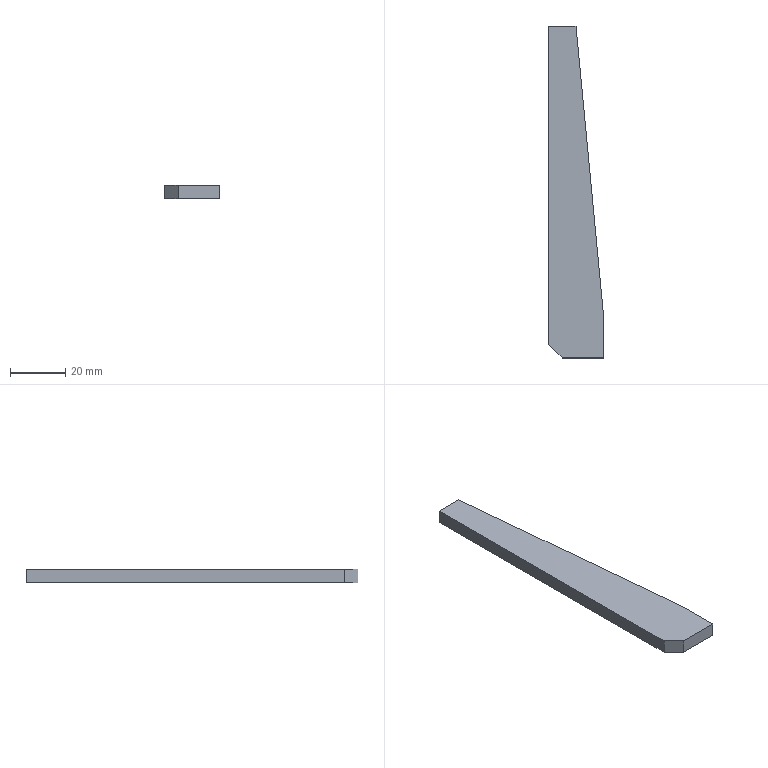Part | SolidWorks | features Chamfer 1, Extrusion 1 | 1 solid | 8 faces | box 20 x 120 x 5 mm | volume 9312 mm3 | plane 8
STEP:
#1=CARTESIAN_POINT('',(5.,0.,5.));
#2=VERTEX_POINT('',#1);
#3=CARTESIAN_POINT('',(20.,0.,5.));
#4=VERTEX_POINT('',#3);
#5=CARTESIAN_POINT('',(20.,0.,5.));
#6=DIRECTION('',(1.,0.,0.));
#7=VECTOR('',#6,1000.);
#8=LINE('',#5,#7);
#9=EDGE_CURVE('',#2,#4,#8,.T.);
#10=ORIENTED_EDGE('',*,*,#9,.F.);
#11=CARTESIAN_POINT('',(5.,0.,0.));
#12=VERTEX_POINT('',#11);
#13=CARTESIAN_POINT('',(5.,0.,5.));
#14=DIRECTION('',(0.,0.,-1.));
#15=VECTOR('',#14,1000.);
#16=LINE('',#13,#15);
#17=EDGE_CURVE('',#2,#12,#16,.T.);
#18=ORIENTED_EDGE('',*,*,#17,.T.);
#19=CARTESIAN_POINT('',(20.,0.,0.));
#20=VERTEX_POINT('',#19);
#21=CARTESIAN_POINT('',(20.,0.,0.));
#22=DIRECTION('',(1.,0.,0.));
#23=VECTOR('',#22,1000.);
#24=LINE('',#21,#23);
#25=EDGE_CURVE('',#12,#20,#24,.T.);
#26=ORIENTED_EDGE('',*,*,#25,.T.);
#27=CARTESIAN_POINT('',(20.,0.,5.));
#28=DIRECTION('',(0.,0.,-1.));
#29=VECTOR('',#28,1000.);
#30=LINE('',#27,#29);
#31=EDGE_CURVE('',#4,#20,#30,.T.);
#32=ORIENTED_EDGE('',*,*,#31,.F.);
#33=EDGE_LOOP('',(#10,#18,#26,#32));
#34=FACE_OUTER_BOUND('',#33,.T.);
#35=CARTESIAN_POINT('',(20.,0.,5.));
#36=DIRECTION('',(0.,1.,0.));
#37=DIRECTION('',(-1.,0.,0.));
#38=AXIS2_PLACEMENT_3D('',#35,#36,#37);
#39=PLANE('',#38);
#40=ADVANCED_FACE('',(#34),#39,.F.);
#41=CARTESIAN_POINT('',(20.,15.,0.));
#42=VERTEX_POINT('',#41);
#43=CARTESIAN_POINT('',(20.,15.,0.));
#44=DIRECTION('',(0.,1.,0.));
#45=VECTOR('',#44,1000.);
#46=LINE('',#43,#45);
#47=EDGE_CURVE('',#20,#42,#46,.T.);
#48=ORIENTED_EDGE('',*,*,#47,.T.);
#49=CARTESIAN_POINT('',(20.,15.,5.));
#50=VERTEX_POINT('',#49);
#51=CARTESIAN_POINT('',(20.,15.,5.));
#52=DIRECTION('',(0.,0.,-1.));
#53=VECTOR('',#52,1000.);
#54=LINE('',#51,#53);
#55=EDGE_CURVE('',#50,#42,#54,.T.);
#56=ORIENTED_EDGE('',*,*,#55,.F.);
#57=CARTESIAN_POINT('',(20.,15.,5.));
#58=DIRECTION('',(0.,1.,0.));
#59=VECTOR('',#58,1000.);
#60=LINE('',#57,#59);
#61=EDGE_CURVE('',#4,#50,#60,.T.);
#62=ORIENTED_EDGE('',*,*,#61,.F.);
#63=ORIENTED_EDGE('',*,*,#31,.T.);
#64=EDGE_LOOP('',(#48,#56,#62,#63));
#65=FACE_OUTER_BOUND('',#64,.T.);
#66=CARTESIAN_POINT('',(20.,15.,5.));
#67=DIRECTION('',(-1.,0.,0.));
#68=DIRECTION('',(0.,0.,1.));
#69=AXIS2_PLACEMENT_3D('',#66,#67,#68);
#70=PLANE('',#69);
#71=ADVANCED_FACE('',(#65),#70,.F.);
#72=CARTESIAN_POINT('',(10.,120.,0.));
#73=VERTEX_POINT('',#72);
#74=CARTESIAN_POINT('',(10.,120.,0.));
#75=DIRECTION('',(-0.09481,0.9955,0.));
#76=VECTOR('',#75,1000.);
#77=LINE('',#74,#76);
#78=EDGE_CURVE('',#42,#73,#77,.T.);
#79=ORIENTED_EDGE('',*,*,#78,.T.);
#80=CARTESIAN_POINT('',(10.,120.,5.));
#81=VERTEX_POINT('',#80);
#82=CARTESIAN_POINT('',(10.,120.,5.));
#83=DIRECTION('',(0.,0.,-1.));
#84=VECTOR('',#83,1000.);
#85=LINE('',#82,#84);
#86=EDGE_CURVE('',#81,#73,#85,.T.);
#87=ORIENTED_EDGE('',*,*,#86,.F.);
#88=CARTESIAN_POINT('',(10.,120.,5.));
#89=DIRECTION('',(-0.09481,0.9955,0.));
#90=VECTOR('',#89,1000.);
#91=LINE('',#88,#90);
#92=EDGE_CURVE('',#50,#81,#91,.T.);
#93=ORIENTED_EDGE('',*,*,#92,.F.);
#94=ORIENTED_EDGE('',*,*,#55,.T.);
#95=EDGE_LOOP('',(#79,#87,#93,#94));
#96=FACE_OUTER_BOUND('',#95,.T.);
#97=CARTESIAN_POINT('',(10.,120.,5.));
#98=DIRECTION('',(-0.9955,-0.09481,0.));
#99=DIRECTION('',(0.09481,-0.9955,0.));
#100=AXIS2_PLACEMENT_3D('',#97,#98,#99);
#101=PLANE('',#100);
#102=ADVANCED_FACE('',(#96),#101,.F.);
#103=CARTESIAN_POINT('',(0.,120.,0.));
#104=VERTEX_POINT('',#103);
#105=CARTESIAN_POINT('',(0.,120.,0.));
#106=DIRECTION('',(-1.,0.,0.));
#107=VECTOR('',#106,1000.);
#108=LINE('',#105,#107);
#109=EDGE_CURVE('',#73,#104,#108,.T.);
#110=ORIENTED_EDGE('',*,*,#109,.T.);
#111=CARTESIAN_POINT('',(0.,120.,5.));
#112=VERTEX_POINT('',#111);
#113=CARTESIAN_POINT('',(0.,120.,5.));
#114=DIRECTION('',(0.,0.,-1.));
#115=VECTOR('',#114,1000.);
#116=LINE('',#113,#115);
#117=EDGE_CURVE('',#112,#104,#116,.T.);
#118=ORIENTED_EDGE('',*,*,#117,.F.);
#119=CARTESIAN_POINT('',(0.,120.,5.));
#120=DIRECTION('',(-1.,0.,0.));
#121=VECTOR('',#120,1000.);
#122=LINE('',#119,#121);
#123=EDGE_CURVE('',#81,#112,#122,.T.);
#124=ORIENTED_EDGE('',*,*,#123,.F.);
#125=ORIENTED_EDGE('',*,*,#86,.T.);
#126=EDGE_LOOP('',(#110,#118,#124,#125));
#127=FACE_OUTER_BOUND('',#126,.T.);
#128=CARTESIAN_POINT('',(0.,120.,5.));
#129=DIRECTION('',(0.,-1.,0.));
#130=DIRECTION('',(0.,0.,-1.));
#131=AXIS2_PLACEMENT_3D('',#128,#129,#130);
#132=PLANE('',#131);
#133=ADVANCED_FACE('',(#127),#132,.F.);
#134=CARTESIAN_POINT('',(0.,5.,0.));
#135=VERTEX_POINT('',#134);
#136=CARTESIAN_POINT('',(0.,0.,0.));
#137=DIRECTION('',(0.,-1.,0.));
#138=VECTOR('',#137,1000.);
#139=LINE('',#136,#138);
#140=EDGE_CURVE('',#104,#135,#139,.T.);
#141=ORIENTED_EDGE('',*,*,#140,.T.);
#142=CARTESIAN_POINT('',(0.,5.,5.));
#143=VERTEX_POINT('',#142);
#144=CARTESIAN_POINT('',(0.,5.,5.));
#145=DIRECTION('',(0.,0.,1.));
#146=VECTOR('',#145,1000.);
#147=LINE('',#144,#146);
#148=EDGE_CURVE('',#135,#143,#147,.T.);
#149=ORIENTED_EDGE('',*,*,#148,.T.);
#150=CARTESIAN_POINT('',(0.,0.,5.));
#151=DIRECTION('',(0.,-1.,0.));
#152=VECTOR('',#151,1000.);
#153=LINE('',#150,#152);
#154=EDGE_CURVE('',#112,#143,#153,.T.);
#155=ORIENTED_EDGE('',*,*,#154,.F.);
#156=ORIENTED_EDGE('',*,*,#117,.T.);
#157=EDGE_LOOP('',(#141,#149,#155,#156));
#158=FACE_OUTER_BOUND('',#157,.T.);
#159=CARTESIAN_POINT('',(0.,0.,5.));
#160=DIRECTION('',(1.,0.,0.));
#161=DIRECTION('',(0.,0.,-1.));
#162=AXIS2_PLACEMENT_3D('',#159,#160,#161);
#163=PLANE('',#162);
#164=ADVANCED_FACE('',(#158),#163,.F.);
#165=ORIENTED_EDGE('',*,*,#154,.T.);
#166=CARTESIAN_POINT('',(5.,0.,5.));
#167=DIRECTION('',(0.7071,-0.7071,0.));
#168=VECTOR('',#167,1000.);
#169=LINE('',#166,#168);
#170=EDGE_CURVE('',#143,#2,#169,.T.);
#171=ORIENTED_EDGE('',*,*,#170,.T.);
#172=ORIENTED_EDGE('',*,*,#9,.T.);
#173=ORIENTED_EDGE('',*,*,#61,.T.);
#174=ORIENTED_EDGE('',*,*,#92,.T.);
#175=ORIENTED_EDGE('',*,*,#123,.T.);
#176=EDGE_LOOP('',(#165,#171,#172,#173,#174,#175));
#177=FACE_OUTER_BOUND('',#176,.T.);
#178=CARTESIAN_POINT('',(0.,0.,5.));
#179=DIRECTION('',(0.,0.,-1.));
#180=DIRECTION('',(-1.,0.,0.));
#181=AXIS2_PLACEMENT_3D('',#178,#179,#180);
#182=PLANE('',#181);
#183=ADVANCED_FACE('',(#177),#182,.F.);
#184=ORIENTED_EDGE('',*,*,#25,.F.);
#185=CARTESIAN_POINT('',(2.5,2.5,0.));
#186=DIRECTION('',(-0.7071,0.7071,0.));
#187=VECTOR('',#186,1000.);
#188=LINE('',#185,#187);
#189=EDGE_CURVE('',#12,#135,#188,.T.);
#190=ORIENTED_EDGE('',*,*,#189,.T.);
#191=ORIENTED_EDGE('',*,*,#140,.F.);
#192=ORIENTED_EDGE('',*,*,#109,.F.);
#193=ORIENTED_EDGE('',*,*,#78,.F.);
#194=ORIENTED_EDGE('',*,*,#47,.F.);
#195=EDGE_LOOP('',(#184,#190,#191,#192,#193,#194));
#196=FACE_OUTER_BOUND('',#195,.T.);
#197=CARTESIAN_POINT('',(0.,0.,0.));
#198=DIRECTION('',(0.,0.,-1.));
#199=DIRECTION('',(-1.,0.,0.));
#200=AXIS2_PLACEMENT_3D('',#197,#198,#199);
#201=PLANE('',#200);
#202=ADVANCED_FACE('',(#196),#201,.T.);
#203=ORIENTED_EDGE('',*,*,#170,.F.);
#204=ORIENTED_EDGE('',*,*,#148,.F.);
#205=ORIENTED_EDGE('',*,*,#189,.F.);
#206=ORIENTED_EDGE('',*,*,#17,.F.);
#207=EDGE_LOOP('',(#203,#204,#205,#206));
#208=FACE_OUTER_BOUND('',#207,.T.);
#209=CARTESIAN_POINT('',(5.,0.,5.));
#210=DIRECTION('',(0.7071,0.7071,0.));
#211=DIRECTION('',(0.,0.,-1.));
#212=AXIS2_PLACEMENT_3D('',#209,#210,#211);
#213=PLANE('',#212);
#214=ADVANCED_FACE('',(#208),#213,.F.);
#215=CLOSED_SHELL('',(#40,#71,#102,#133,#164,#183,#202,#214));
#216=MANIFOLD_SOLID_BREP('',#215);
#217=CARTESIAN_POINT('',(0.,0.,0.));
#218=DIRECTION('',(0.,0.,1.));
#219=DIRECTION('',(1.,0.,0.));
#220=AXIS2_PLACEMENT_3D('',#217,#218,#219);
#221=(LENGTH_UNIT()NAMED_UNIT(*)SI_UNIT(.MILLI.,.METRE.));
#222=UNCERTAINTY_MEASURE_WITH_UNIT(LENGTH_MEASURE(0.00001),#221,'','');
#223=(NAMED_UNIT(*)PLANE_ANGLE_UNIT()SI_UNIT($,.RADIAN.));
#224=(NAMED_UNIT(*)SI_UNIT($,.STERADIAN.)SOLID_ANGLE_UNIT());
#225=(GEOMETRIC_REPRESENTATION_CONTEXT(3)GLOBAL_UNCERTAINTY_ASSIGNED_CONTEXT((#222))GLOBAL_UNIT_ASSIGNED_CONTEXT((#221,#223,#224))REPRESENTATION_CONTEXT('',''));
#226=ADVANCED_BREP_SHAPE_REPRESENTATION('',(#216,#220),#225);